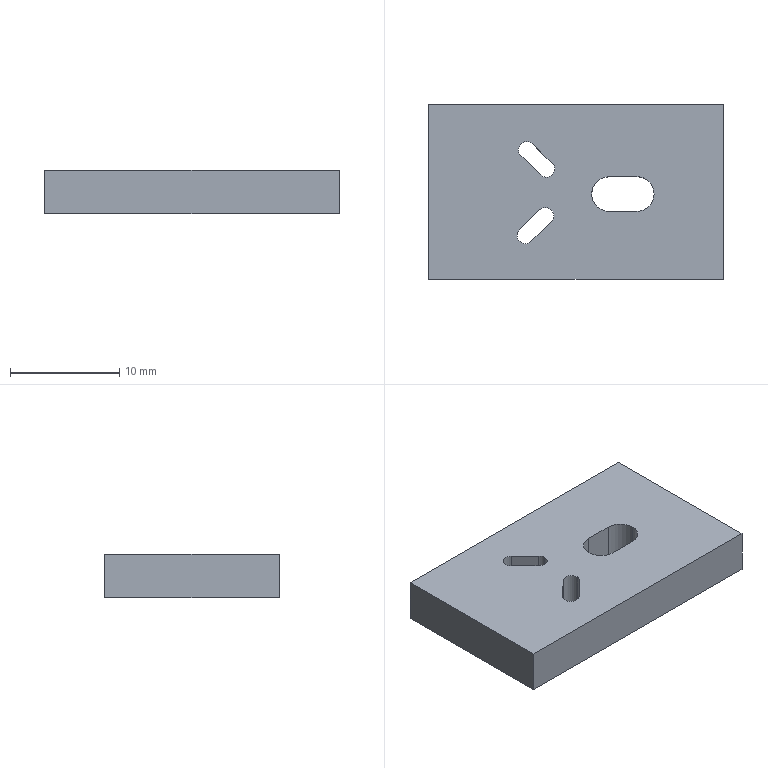Part | SolidWorks | features Cut 2, Extrusion 1 | 1 solid | 21 faces | box 27 x 16 x 4 mm | volume 1619 mm3 | plane 12 | cylinder 9 | commonest cylinder face diameters 1.5 x6 3.18 x3
STEP:
#1=CARTESIAN_POINT('',(9.464,-2.48,0.));
#2=VERTEX_POINT('',#1);
#3=CARTESIAN_POINT('',(11.055,-4.07,0.));
#4=VERTEX_POINT('',#3);
#5=CARTESIAN_POINT('',(9.465,-4.07,0.));
#6=DIRECTION('',(0.,0.,-1.));
#7=DIRECTION('',(1.,0.,0.));
#8=AXIS2_PLACEMENT_3D('',#5,#6,#7);
#9=CIRCLE('',#8,1.59);
#10=EDGE_CURVE('',#2,#4,#9,.T.);
#11=ORIENTED_EDGE('',*,*,#10,.T.);
#12=CARTESIAN_POINT('',(11.055,-4.07,4.));
#13=VERTEX_POINT('',#12);
#14=CARTESIAN_POINT('',(11.055,-4.07,-4.497));
#15=DIRECTION('',(0.,0.,1.));
#16=VECTOR('',#15,1000.);
#17=LINE('',#14,#16);
#18=EDGE_CURVE('',#4,#13,#17,.T.);
#19=ORIENTED_EDGE('',*,*,#18,.T.);
#20=CARTESIAN_POINT('',(9.464,-2.48,4.));
#21=VERTEX_POINT('',#20);
#22=CARTESIAN_POINT('',(9.465,-4.07,4.));
#23=DIRECTION('',(0.,0.,1.));
#24=DIRECTION('',(1.,0.,0.));
#25=AXIS2_PLACEMENT_3D('',#22,#23,#24);
#26=CIRCLE('',#25,1.59);
#27=EDGE_CURVE('',#13,#21,#26,.T.);
#28=ORIENTED_EDGE('',*,*,#27,.T.);
#29=CARTESIAN_POINT('',(9.464,-2.48,-5.208));
#30=DIRECTION('',(0.,0.,1.));
#31=VECTOR('',#30,1000.);
#32=LINE('',#29,#31);
#33=EDGE_CURVE('',#2,#21,#32,.T.);
#34=ORIENTED_EDGE('',*,*,#33,.F.);
#35=EDGE_LOOP('',(#11,#19,#28,#34));
#36=FACE_OUTER_BOUND('',#35,.T.);
#37=CARTESIAN_POINT('',(9.465,-4.07,-4.497));
#38=DIRECTION('',(0.,0.,1.));
#39=DIRECTION('',(1.,0.,0.));
#40=AXIS2_PLACEMENT_3D('',#37,#38,#39);
#41=CYLINDRICAL_SURFACE('',#40,1.59);
#42=ADVANCED_FACE('',(#36),#41,.F.);
#43=CARTESIAN_POINT('',(1.721,-1.242,0.));
#44=VERTEX_POINT('',#43);
#45=CARTESIAN_POINT('',(1.95,-1.782,0.));
#46=VERTEX_POINT('',#45);
#47=CARTESIAN_POINT('',(1.2,-1.782,0.));
#48=DIRECTION('',(0.,0.,-1.));
#49=DIRECTION('',(1.,0.,0.));
#50=AXIS2_PLACEMENT_3D('',#47,#48,#49);
#51=CIRCLE('',#50,0.75);
#52=EDGE_CURVE('',#44,#46,#51,.T.);
#53=ORIENTED_EDGE('',*,*,#52,.T.);
#54=CARTESIAN_POINT('',(1.95,-1.782,4.));
#55=VERTEX_POINT('',#54);
#56=CARTESIAN_POINT('',(1.95,-1.782,-4.497));
#57=DIRECTION('',(0.,0.,1.));
#58=VECTOR('',#57,1000.);
#59=LINE('',#56,#58);
#60=EDGE_CURVE('',#46,#55,#59,.T.);
#61=ORIENTED_EDGE('',*,*,#60,.T.);
#62=CARTESIAN_POINT('',(1.721,-1.242,4.));
#63=VERTEX_POINT('',#62);
#64=CARTESIAN_POINT('',(1.2,-1.782,4.));
#65=DIRECTION('',(0.,0.,1.));
#66=DIRECTION('',(1.,0.,0.));
#67=AXIS2_PLACEMENT_3D('',#64,#65,#66);
#68=CIRCLE('',#67,0.75);
#69=EDGE_CURVE('',#55,#63,#68,.T.);
#70=ORIENTED_EDGE('',*,*,#69,.T.);
#71=CARTESIAN_POINT('',(1.721,-1.242,-5.208));
#72=DIRECTION('',(0.,0.,1.));
#73=VECTOR('',#72,1000.);
#74=LINE('',#71,#73);
#75=EDGE_CURVE('',#44,#63,#74,.T.);
#76=ORIENTED_EDGE('',*,*,#75,.F.);
#77=EDGE_LOOP('',(#53,#61,#70,#76));
#78=FACE_OUTER_BOUND('',#77,.T.);
#79=CARTESIAN_POINT('',(1.2,-1.782,-4.497));
#80=DIRECTION('',(0.,0.,1.));
#81=DIRECTION('',(1.,0.,0.));
#82=AXIS2_PLACEMENT_3D('',#79,#80,#81);
#83=CYLINDRICAL_SURFACE('',#82,0.75);
#84=ADVANCED_FACE('',(#78),#83,.F.);
#85=CARTESIAN_POINT('',(0.6012,-5.518,0.));
#86=VERTEX_POINT('',#85);
#87=CARTESIAN_POINT('',(1.873,-6.057,0.));
#88=VERTEX_POINT('',#87);
#89=CARTESIAN_POINT('',(1.123,-6.057,0.));
#90=DIRECTION('',(0.,0.,-1.));
#91=DIRECTION('',(1.,0.,0.));
#92=AXIS2_PLACEMENT_3D('',#89,#90,#91);
#93=CIRCLE('',#92,0.75);
#94=EDGE_CURVE('',#86,#88,#93,.T.);
#95=ORIENTED_EDGE('',*,*,#94,.T.);
#96=CARTESIAN_POINT('',(1.873,-6.057,4.));
#97=VERTEX_POINT('',#96);
#98=CARTESIAN_POINT('',(1.873,-6.057,-4.497));
#99=DIRECTION('',(0.,0.,1.));
#100=VECTOR('',#99,1000.);
#101=LINE('',#98,#100);
#102=EDGE_CURVE('',#88,#97,#101,.T.);
#103=ORIENTED_EDGE('',*,*,#102,.T.);
#104=CARTESIAN_POINT('',(0.6012,-5.518,4.));
#105=VERTEX_POINT('',#104);
#106=CARTESIAN_POINT('',(1.123,-6.057,4.));
#107=DIRECTION('',(0.,0.,1.));
#108=DIRECTION('',(1.,0.,0.));
#109=AXIS2_PLACEMENT_3D('',#106,#107,#108);
#110=CIRCLE('',#109,0.75);
#111=EDGE_CURVE('',#97,#105,#110,.T.);
#112=ORIENTED_EDGE('',*,*,#111,.T.);
#113=CARTESIAN_POINT('',(0.6012,-5.518,-5.208));
#114=DIRECTION('',(0.,0.,1.));
#115=VECTOR('',#114,1000.);
#116=LINE('',#113,#115);
#117=EDGE_CURVE('',#86,#105,#116,.T.);
#118=ORIENTED_EDGE('',*,*,#117,.F.);
#119=EDGE_LOOP('',(#95,#103,#112,#118));
#120=FACE_OUTER_BOUND('',#119,.T.);
#121=CARTESIAN_POINT('',(1.123,-6.057,-4.497));
#122=DIRECTION('',(0.,0.,1.));
#123=DIRECTION('',(1.,0.,0.));
#124=AXIS2_PLACEMENT_3D('',#121,#122,#123);
#125=CYLINDRICAL_SURFACE('',#124,0.75);
#126=ADVANCED_FACE('',(#120),#125,.F.);
#127=ORIENTED_EDGE('',*,*,#102,.F.);
#128=CARTESIAN_POINT('',(1.644,-6.596,0.));
#129=VERTEX_POINT('',#128);
#130=CARTESIAN_POINT('',(1.123,-6.057,0.));
#131=DIRECTION('',(0.,0.,-1.));
#132=DIRECTION('',(1.,0.,0.));
#133=AXIS2_PLACEMENT_3D('',#130,#131,#132);
#134=CIRCLE('',#133,0.75);
#135=EDGE_CURVE('',#88,#129,#134,.T.);
#136=ORIENTED_EDGE('',*,*,#135,.T.);
#137=CARTESIAN_POINT('',(1.644,-6.596,4.));
#138=VERTEX_POINT('',#137);
#139=CARTESIAN_POINT('',(1.644,-6.596,-5.208));
#140=DIRECTION('',(0.,0.,1.));
#141=VECTOR('',#140,1000.);
#142=LINE('',#139,#141);
#143=EDGE_CURVE('',#129,#138,#142,.T.);
#144=ORIENTED_EDGE('',*,*,#143,.T.);
#145=CARTESIAN_POINT('',(1.123,-6.057,4.));
#146=DIRECTION('',(0.,0.,1.));
#147=DIRECTION('',(1.,0.,0.));
#148=AXIS2_PLACEMENT_3D('',#145,#146,#147);
#149=CIRCLE('',#148,0.75);
#150=EDGE_CURVE('',#138,#97,#149,.T.);
#151=ORIENTED_EDGE('',*,*,#150,.T.);
#152=EDGE_LOOP('',(#127,#136,#144,#151));
#153=FACE_OUTER_BOUND('',#152,.T.);
#154=CARTESIAN_POINT('',(1.123,-6.057,-4.497));
#155=DIRECTION('',(0.,0.,1.));
#156=DIRECTION('',(1.,0.,0.));
#157=AXIS2_PLACEMENT_3D('',#154,#155,#156);
#158=CYLINDRICAL_SURFACE('',#157,0.75);
#159=ADVANCED_FACE('',(#153),#158,.F.);
#160=CARTESIAN_POINT('',(-9.601,4.118,0.));
#161=VERTEX_POINT('',#160);
#162=CARTESIAN_POINT('',(-9.601,-11.882,0.));
#163=VERTEX_POINT('',#162);
#164=CARTESIAN_POINT('',(-9.601,4.118,0.));
#165=DIRECTION('',(0.,-1.,0.));
#166=VECTOR('',#165,1000.);
#167=LINE('',#164,#166);
#168=EDGE_CURVE('',#161,#163,#167,.T.);
#169=ORIENTED_EDGE('',*,*,#168,.T.);
#170=CARTESIAN_POINT('',(-9.601,-11.882,4.));
#171=VERTEX_POINT('',#170);
#172=CARTESIAN_POINT('',(-9.601,-11.882,4.));
#173=DIRECTION('',(0.,0.,-1.));
#174=VECTOR('',#173,1000.);
#175=LINE('',#172,#174);
#176=EDGE_CURVE('',#171,#163,#175,.T.);
#177=ORIENTED_EDGE('',*,*,#176,.F.);
#178=CARTESIAN_POINT('',(-9.601,4.118,4.));
#179=VERTEX_POINT('',#178);
#180=CARTESIAN_POINT('',(-9.601,4.118,4.));
#181=DIRECTION('',(0.,-1.,0.));
#182=VECTOR('',#181,1000.);
#183=LINE('',#180,#182);
#184=EDGE_CURVE('',#179,#171,#183,.T.);
#185=ORIENTED_EDGE('',*,*,#184,.F.);
#186=CARTESIAN_POINT('',(-9.601,4.118,4.));
#187=DIRECTION('',(0.,0.,-1.));
#188=VECTOR('',#187,1000.);
#189=LINE('',#186,#188);
#190=EDGE_CURVE('',#179,#161,#189,.T.);
#191=ORIENTED_EDGE('',*,*,#190,.T.);
#192=EDGE_LOOP('',(#169,#177,#185,#191));
#193=FACE_OUTER_BOUND('',#192,.T.);
#194=CARTESIAN_POINT('',(-9.601,4.118,4.));
#195=DIRECTION('',(1.,0.,0.));
#196=DIRECTION('',(0.,1.,0.));
#197=AXIS2_PLACEMENT_3D('',#194,#195,#196);
#198=PLANE('',#197);
#199=ADVANCED_FACE('',(#193),#198,.F.);
#200=CARTESIAN_POINT('',(17.399,-11.882,0.));
#201=VERTEX_POINT('',#200);
#202=CARTESIAN_POINT('',(-9.601,-11.882,0.));
#203=DIRECTION('',(1.,0.,0.));
#204=VECTOR('',#203,1000.);
#205=LINE('',#202,#204);
#206=EDGE_CURVE('',#163,#201,#205,.T.);
#207=ORIENTED_EDGE('',*,*,#206,.T.);
#208=CARTESIAN_POINT('',(17.399,-11.882,4.));
#209=VERTEX_POINT('',#208);
#210=CARTESIAN_POINT('',(17.399,-11.882,4.));
#211=DIRECTION('',(0.,0.,-1.));
#212=VECTOR('',#211,1000.);
#213=LINE('',#210,#212);
#214=EDGE_CURVE('',#209,#201,#213,.T.);
#215=ORIENTED_EDGE('',*,*,#214,.F.);
#216=CARTESIAN_POINT('',(-9.601,-11.882,4.));
#217=DIRECTION('',(1.,0.,0.));
#218=VECTOR('',#217,1000.);
#219=LINE('',#216,#218);
#220=EDGE_CURVE('',#171,#209,#219,.T.);
#221=ORIENTED_EDGE('',*,*,#220,.F.);
#222=ORIENTED_EDGE('',*,*,#176,.T.);
#223=EDGE_LOOP('',(#207,#215,#221,#222));
#224=FACE_OUTER_BOUND('',#223,.T.);
#225=CARTESIAN_POINT('',(-9.601,-11.882,4.));
#226=DIRECTION('',(0.,1.,0.));
#227=DIRECTION('',(0.,0.,1.));
#228=AXIS2_PLACEMENT_3D('',#225,#226,#227);
#229=PLANE('',#228);
#230=ADVANCED_FACE('',(#224),#229,.F.);
#231=CARTESIAN_POINT('',(17.399,4.118,0.));
#232=VERTEX_POINT('',#231);
#233=CARTESIAN_POINT('',(17.399,4.118,0.));
#234=DIRECTION('',(0.,1.,0.));
#235=VECTOR('',#234,1000.);
#236=LINE('',#233,#235);
#237=EDGE_CURVE('',#201,#232,#236,.T.);
#238=ORIENTED_EDGE('',*,*,#237,.T.);
#239=CARTESIAN_POINT('',(17.399,4.118,4.));
#240=VERTEX_POINT('',#239);
#241=CARTESIAN_POINT('',(17.399,4.118,4.));
#242=DIRECTION('',(0.,0.,-1.));
#243=VECTOR('',#242,1000.);
#244=LINE('',#241,#243);
#245=EDGE_CURVE('',#240,#232,#244,.T.);
#246=ORIENTED_EDGE('',*,*,#245,.F.);
#247=CARTESIAN_POINT('',(17.399,4.118,4.));
#248=DIRECTION('',(0.,1.,0.));
#249=VECTOR('',#248,1000.);
#250=LINE('',#247,#249);
#251=EDGE_CURVE('',#209,#240,#250,.T.);
#252=ORIENTED_EDGE('',*,*,#251,.F.);
#253=ORIENTED_EDGE('',*,*,#214,.T.);
#254=EDGE_LOOP('',(#238,#246,#252,#253));
#255=FACE_OUTER_BOUND('',#254,.T.);
#256=CARTESIAN_POINT('',(17.399,4.118,4.));
#257=DIRECTION('',(-1.,0.,0.));
#258=DIRECTION('',(0.,-1.,0.));
#259=AXIS2_PLACEMENT_3D('',#256,#257,#258);
#260=PLANE('',#259);
#261=ADVANCED_FACE('',(#255),#260,.F.);
#262=CARTESIAN_POINT('',(-9.601,4.118,0.));
#263=DIRECTION('',(-1.,0.,0.));
#264=VECTOR('',#263,1000.);
#265=LINE('',#262,#264);
#266=EDGE_CURVE('',#232,#161,#265,.T.);
#267=ORIENTED_EDGE('',*,*,#266,.T.);
#268=ORIENTED_EDGE('',*,*,#190,.F.);
#269=CARTESIAN_POINT('',(-9.601,4.118,4.));
#270=DIRECTION('',(-1.,0.,0.));
#271=VECTOR('',#270,1000.);
#272=LINE('',#269,#271);
#273=EDGE_CURVE('',#240,#179,#272,.T.);
#274=ORIENTED_EDGE('',*,*,#273,.F.);
#275=ORIENTED_EDGE('',*,*,#245,.T.);
#276=EDGE_LOOP('',(#267,#268,#274,#275));
#277=FACE_OUTER_BOUND('',#276,.T.);
#278=CARTESIAN_POINT('',(-9.601,4.118,4.));
#279=DIRECTION('',(0.,-1.,0.));
#280=DIRECTION('',(0.,0.,-1.));
#281=AXIS2_PLACEMENT_3D('',#278,#279,#280);
#282=PLANE('',#281);
#283=ADVANCED_FACE('',(#277),#282,.F.);
#284=CARTESIAN_POINT('',(-0.1034,0.5215,4.));
#285=VERTEX_POINT('',#284);
#286=CARTESIAN_POINT('',(1.721,-1.242,4.));
#287=DIRECTION('',(-0.719,0.695,0.));
#288=VECTOR('',#287,1000.);
#289=LINE('',#286,#288);
#290=EDGE_CURVE('',#63,#285,#289,.T.);
#291=ORIENTED_EDGE('',*,*,#290,.F.);
#292=ORIENTED_EDGE('',*,*,#69,.F.);
#293=CARTESIAN_POINT('',(0.6786,-2.321,4.));
#294=VERTEX_POINT('',#293);
#295=CARTESIAN_POINT('',(1.2,-1.782,4.));
#296=DIRECTION('',(0.,0.,1.));
#297=DIRECTION('',(1.,0.,0.));
#298=AXIS2_PLACEMENT_3D('',#295,#296,#297);
#299=CIRCLE('',#298,0.75);
#300=EDGE_CURVE('',#294,#55,#299,.T.);
#301=ORIENTED_EDGE('',*,*,#300,.F.);
#302=CARTESIAN_POINT('',(-1.146,-0.5569,4.));
#303=VERTEX_POINT('',#302);
#304=CARTESIAN_POINT('',(-1.146,-0.5569,4.));
#305=DIRECTION('',(0.719,-0.695,0.));
#306=VECTOR('',#305,1000.);
#307=LINE('',#304,#306);
#308=EDGE_CURVE('',#303,#294,#307,.T.);
#309=ORIENTED_EDGE('',*,*,#308,.F.);
#310=CARTESIAN_POINT('',(-0.6247,-0.01768,4.));
#311=DIRECTION('',(0.,0.,1.));
#312=DIRECTION('',(1.,0.,0.));
#313=AXIS2_PLACEMENT_3D('',#310,#311,#312);
#314=CIRCLE('',#313,0.75);
#315=EDGE_CURVE('',#285,#303,#314,.T.);
#316=ORIENTED_EDGE('',*,*,#315,.F.);
#317=EDGE_LOOP('',(#291,#292,#301,#309,#316));
#318=FACE_BOUND('',#317,.T.);
#319=CARTESIAN_POINT('',(6.932,-2.481,4.));
#320=VERTEX_POINT('',#319);
#321=CARTESIAN_POINT('',(6.932,-2.481,4.));
#322=DIRECTION('',(-1.,-0.0007677,0.));
#323=VECTOR('',#322,1000.);
#324=LINE('',#321,#323);
#325=EDGE_CURVE('',#21,#320,#324,.T.);
#326=ORIENTED_EDGE('',*,*,#325,.F.);
#327=ORIENTED_EDGE('',*,*,#27,.F.);
#328=CARTESIAN_POINT('',(9.467,-5.66,4.));
#329=VERTEX_POINT('',#328);
#330=CARTESIAN_POINT('',(9.465,-4.07,4.));
#331=DIRECTION('',(0.,0.,1.));
#332=DIRECTION('',(1.,0.,0.));
#333=AXIS2_PLACEMENT_3D('',#330,#331,#332);
#334=CIRCLE('',#333,1.59);
#335=EDGE_CURVE('',#329,#13,#334,.T.);
#336=ORIENTED_EDGE('',*,*,#335,.F.);
#337=CARTESIAN_POINT('',(6.934,-5.661,4.));
#338=VERTEX_POINT('',#337);
#339=CARTESIAN_POINT('',(6.934,-5.661,4.));
#340=DIRECTION('',(1.,0.0007677,0.));
#341=VECTOR('',#340,1000.);
#342=LINE('',#339,#341);
#343=EDGE_CURVE('',#338,#329,#342,.T.);
#344=ORIENTED_EDGE('',*,*,#343,.F.);
#345=CARTESIAN_POINT('',(6.933,-4.071,4.));
#346=DIRECTION('',(0.,0.,1.));
#347=DIRECTION('',(1.,0.,0.));
#348=AXIS2_PLACEMENT_3D('',#345,#346,#347);
#349=CIRCLE('',#348,1.59);
#350=EDGE_CURVE('',#320,#338,#349,.T.);
#351=ORIENTED_EDGE('',*,*,#350,.F.);
#352=EDGE_LOOP('',(#326,#327,#336,#344,#351));
#353=FACE_BOUND('',#352,.T.);
#354=CARTESIAN_POINT('',(-0.2339,-8.411,4.));
#355=VERTEX_POINT('',#354);
#356=CARTESIAN_POINT('',(1.644,-6.596,4.));
#357=DIRECTION('',(0.719,0.695,0.));
#358=VECTOR('',#357,1000.);
#359=LINE('',#356,#358);
#360=EDGE_CURVE('',#355,#138,#359,.T.);
#361=ORIENTED_EDGE('',*,*,#360,.F.);
#362=CARTESIAN_POINT('',(-1.276,-7.333,4.));
#363=VERTEX_POINT('',#362);
#364=CARTESIAN_POINT('',(-0.7552,-7.872,4.));
#365=DIRECTION('',(0.,0.,1.));
#366=DIRECTION('',(1.,0.,0.));
#367=AXIS2_PLACEMENT_3D('',#364,#365,#366);
#368=CIRCLE('',#367,0.75);
#369=EDGE_CURVE('',#363,#355,#368,.T.);
#370=ORIENTED_EDGE('',*,*,#369,.F.);
#371=CARTESIAN_POINT('',(-1.276,-7.333,4.));
#372=DIRECTION('',(-0.719,-0.695,0.));
#373=VECTOR('',#372,1000.);
#374=LINE('',#371,#373);
#375=EDGE_CURVE('',#105,#363,#374,.T.);
#376=ORIENTED_EDGE('',*,*,#375,.F.);
#377=ORIENTED_EDGE('',*,*,#111,.F.);
#378=ORIENTED_EDGE('',*,*,#150,.F.);
#379=EDGE_LOOP('',(#361,#370,#376,#377,#378));
#380=FACE_BOUND('',#379,.T.);
#381=ORIENTED_EDGE('',*,*,#184,.T.);
#382=ORIENTED_EDGE('',*,*,#220,.T.);
#383=ORIENTED_EDGE('',*,*,#251,.T.);
#384=ORIENTED_EDGE('',*,*,#273,.T.);
#385=EDGE_LOOP('',(#381,#382,#383,#384));
#386=FACE_OUTER_BOUND('',#385,.T.);
#387=CARTESIAN_POINT('',(0.,0.,4.));
#388=DIRECTION('',(0.,0.,1.));
#389=DIRECTION('',(1.,0.,0.));
#390=AXIS2_PLACEMENT_3D('',#387,#388,#389);
#391=PLANE('',#390);
#392=ADVANCED_FACE('',(#318,#353,#380,#386),#391,.T.);
#393=ORIENTED_EDGE('',*,*,#10,.F.);
#394=CARTESIAN_POINT('',(6.932,-2.481,0.));
#395=VERTEX_POINT('',#394);
#396=CARTESIAN_POINT('',(6.932,-2.481,0.));
#397=DIRECTION('',(1.,0.0007677,0.));
#398=VECTOR('',#397,1000.);
#399=LINE('',#396,#398);
#400=EDGE_CURVE('',#395,#2,#399,.T.);
#401=ORIENTED_EDGE('',*,*,#400,.F.);
#402=CARTESIAN_POINT('',(6.934,-5.661,0.));
#403=VERTEX_POINT('',#402);
#404=CARTESIAN_POINT('',(6.933,-4.071,0.));
#405=DIRECTION('',(0.,0.,-1.));
#406=DIRECTION('',(1.,0.,0.));
#407=AXIS2_PLACEMENT_3D('',#404,#405,#406);
#408=CIRCLE('',#407,1.59);
#409=EDGE_CURVE('',#403,#395,#408,.T.);
#410=ORIENTED_EDGE('',*,*,#409,.F.);
#411=CARTESIAN_POINT('',(9.467,-5.66,0.));
#412=VERTEX_POINT('',#411);
#413=CARTESIAN_POINT('',(6.934,-5.661,0.));
#414=DIRECTION('',(-1.,-0.0007677,0.));
#415=VECTOR('',#414,1000.);
#416=LINE('',#413,#415);
#417=EDGE_CURVE('',#412,#403,#416,.T.);
#418=ORIENTED_EDGE('',*,*,#417,.F.);
#419=CARTESIAN_POINT('',(9.465,-4.07,0.));
#420=DIRECTION('',(0.,0.,-1.));
#421=DIRECTION('',(1.,0.,0.));
#422=AXIS2_PLACEMENT_3D('',#419,#420,#421);
#423=CIRCLE('',#422,1.59);
#424=EDGE_CURVE('',#4,#412,#423,.T.);
#425=ORIENTED_EDGE('',*,*,#424,.F.);
#426=EDGE_LOOP('',(#393,#401,#410,#418,#425));
#427=FACE_BOUND('',#426,.T.);
#428=CARTESIAN_POINT('',(-0.2339,-8.411,0.));
#429=VERTEX_POINT('',#428);
#430=CARTESIAN_POINT('',(-1.276,-7.333,0.));
#431=VERTEX_POINT('',#430);
#432=CARTESIAN_POINT('',(-0.7552,-7.872,0.));
#433=DIRECTION('',(0.,0.,-1.));
#434=DIRECTION('',(1.,0.,0.));
#435=AXIS2_PLACEMENT_3D('',#432,#433,#434);
#436=CIRCLE('',#435,0.75);
#437=EDGE_CURVE('',#429,#431,#436,.T.);
#438=ORIENTED_EDGE('',*,*,#437,.F.);
#439=CARTESIAN_POINT('',(1.644,-6.596,0.));
#440=DIRECTION('',(-0.719,-0.695,0.));
#441=VECTOR('',#440,1000.);
#442=LINE('',#439,#441);
#443=EDGE_CURVE('',#129,#429,#442,.T.);
#444=ORIENTED_EDGE('',*,*,#443,.F.);
#445=ORIENTED_EDGE('',*,*,#135,.F.);
#446=ORIENTED_EDGE('',*,*,#94,.F.);
#447=CARTESIAN_POINT('',(-1.276,-7.333,0.));
#448=DIRECTION('',(0.719,0.695,0.));
#449=VECTOR('',#448,1000.);
#450=LINE('',#447,#449);
#451=EDGE_CURVE('',#431,#86,#450,.T.);
#452=ORIENTED_EDGE('',*,*,#451,.F.);
#453=EDGE_LOOP('',(#438,#444,#445,#446,#452));
#454=FACE_BOUND('',#453,.T.);
#455=ORIENTED_EDGE('',*,*,#52,.F.);
#456=CARTESIAN_POINT('',(-0.1034,0.5215,0.));
#457=VERTEX_POINT('',#456);
#458=CARTESIAN_POINT('',(1.721,-1.242,0.));
#459=DIRECTION('',(0.719,-0.695,0.));
#460=VECTOR('',#459,1000.);
#461=LINE('',#458,#460);
#462=EDGE_CURVE('',#457,#44,#461,.T.);
#463=ORIENTED_EDGE('',*,*,#462,.F.);
#464=CARTESIAN_POINT('',(-1.146,-0.5569,0.));
#465=VERTEX_POINT('',#464);
#466=CARTESIAN_POINT('',(-0.6247,-0.01768,0.));
#467=DIRECTION('',(0.,0.,-1.));
#468=DIRECTION('',(1.,0.,0.));
#469=AXIS2_PLACEMENT_3D('',#466,#467,#468);
#470=CIRCLE('',#469,0.75);
#471=EDGE_CURVE('',#465,#457,#470,.T.);
#472=ORIENTED_EDGE('',*,*,#471,.F.);
#473=CARTESIAN_POINT('',(0.6786,-2.321,0.));
#474=VERTEX_POINT('',#473);
#475=CARTESIAN_POINT('',(-1.146,-0.5569,0.));
#476=DIRECTION('',(-0.719,0.695,0.));
#477=VECTOR('',#476,1000.);
#478=LINE('',#475,#477);
#479=EDGE_CURVE('',#474,#465,#478,.T.);
#480=ORIENTED_EDGE('',*,*,#479,.F.);
#481=CARTESIAN_POINT('',(1.2,-1.782,0.));
#482=DIRECTION('',(0.,0.,-1.));
#483=DIRECTION('',(1.,0.,0.));
#484=AXIS2_PLACEMENT_3D('',#481,#482,#483);
#485=CIRCLE('',#484,0.75);
#486=EDGE_CURVE('',#46,#474,#485,.T.);
#487=ORIENTED_EDGE('',*,*,#486,.F.);
#488=EDGE_LOOP('',(#455,#463,#472,#480,#487));
#489=FACE_BOUND('',#488,.T.);
#490=ORIENTED_EDGE('',*,*,#168,.F.);
#491=ORIENTED_EDGE('',*,*,#266,.F.);
#492=ORIENTED_EDGE('',*,*,#237,.F.);
#493=ORIENTED_EDGE('',*,*,#206,.F.);
#494=EDGE_LOOP('',(#490,#491,#492,#493));
#495=FACE_OUTER_BOUND('',#494,.T.);
#496=CARTESIAN_POINT('',(0.,0.,0.));
#497=DIRECTION('',(0.,0.,1.));
#498=DIRECTION('',(1.,0.,0.));
#499=AXIS2_PLACEMENT_3D('',#496,#497,#498);
#500=PLANE('',#499);
#501=ADVANCED_FACE('',(#427,#454,#489,#495),#500,.F.);
#502=ORIENTED_EDGE('',*,*,#60,.F.);
#503=ORIENTED_EDGE('',*,*,#486,.T.);
#504=CARTESIAN_POINT('',(0.6786,-2.321,-5.208));
#505=DIRECTION('',(0.,0.,1.));
#506=VECTOR('',#505,1000.);
#507=LINE('',#504,#506);
#508=EDGE_CURVE('',#474,#294,#507,.T.);
#509=ORIENTED_EDGE('',*,*,#508,.T.);
#510=ORIENTED_EDGE('',*,*,#300,.T.);
#511=EDGE_LOOP('',(#502,#503,#509,#510));
#512=FACE_OUTER_BOUND('',#511,.T.);
#513=CARTESIAN_POINT('',(1.2,-1.782,-4.497));
#514=DIRECTION('',(0.,0.,1.));
#515=DIRECTION('',(1.,0.,0.));
#516=AXIS2_PLACEMENT_3D('',#513,#514,#515);
#517=CYLINDRICAL_SURFACE('',#516,0.75);
#518=ADVANCED_FACE('',(#512),#517,.F.);
#519=ORIENTED_EDGE('',*,*,#18,.F.);
#520=ORIENTED_EDGE('',*,*,#424,.T.);
#521=CARTESIAN_POINT('',(9.467,-5.66,-5.208));
#522=DIRECTION('',(0.,0.,1.));
#523=VECTOR('',#522,1000.);
#524=LINE('',#521,#523);
#525=EDGE_CURVE('',#412,#329,#524,.T.);
#526=ORIENTED_EDGE('',*,*,#525,.T.);
#527=ORIENTED_EDGE('',*,*,#335,.T.);
#528=EDGE_LOOP('',(#519,#520,#526,#527));
#529=FACE_OUTER_BOUND('',#528,.T.);
#530=CARTESIAN_POINT('',(9.465,-4.07,-4.497));
#531=DIRECTION('',(0.,0.,1.));
#532=DIRECTION('',(1.,0.,0.));
#533=AXIS2_PLACEMENT_3D('',#530,#531,#532);
#534=CYLINDRICAL_SURFACE('',#533,1.59);
#535=ADVANCED_FACE('',(#529),#534,.F.);
#536=ORIENTED_EDGE('',*,*,#409,.T.);
#537=CARTESIAN_POINT('',(6.932,-2.481,-5.208));
#538=DIRECTION('',(0.,0.,1.));
#539=VECTOR('',#538,1000.);
#540=LINE('',#537,#539);
#541=EDGE_CURVE('',#395,#320,#540,.T.);
#542=ORIENTED_EDGE('',*,*,#541,.T.);
#543=ORIENTED_EDGE('',*,*,#350,.T.);
#544=CARTESIAN_POINT('',(6.934,-5.661,-5.208));
#545=DIRECTION('',(0.,0.,1.));
#546=VECTOR('',#545,1000.);
#547=LINE('',#544,#546);
#548=EDGE_CURVE('',#403,#338,#547,.T.);
#549=ORIENTED_EDGE('',*,*,#548,.F.);
#550=EDGE_LOOP('',(#536,#542,#543,#549));
#551=FACE_OUTER_BOUND('',#550,.T.);
#552=CARTESIAN_POINT('',(6.933,-4.071,-5.208));
#553=DIRECTION('',(0.,0.,1.));
#554=DIRECTION('',(1.,0.,0.));
#555=AXIS2_PLACEMENT_3D('',#552,#553,#554);
#556=CYLINDRICAL_SURFACE('',#555,1.59);
#557=ADVANCED_FACE('',(#551),#556,.F.);
#558=ORIENTED_EDGE('',*,*,#400,.T.);
#559=ORIENTED_EDGE('',*,*,#33,.T.);
#560=ORIENTED_EDGE('',*,*,#325,.T.);
#561=ORIENTED_EDGE('',*,*,#541,.F.);
#562=EDGE_LOOP('',(#558,#559,#560,#561));
#563=FACE_OUTER_BOUND('',#562,.T.);
#564=CARTESIAN_POINT('',(6.932,-2.481,-5.208));
#565=DIRECTION('',(-0.0007677,1.,0.));
#566=DIRECTION('',(-1.,-0.0007677,0.));
#567=AXIS2_PLACEMENT_3D('',#564,#565,#566);
#568=PLANE('',#567);
#569=ADVANCED_FACE('',(#563),#568,.F.);
#570=ORIENTED_EDGE('',*,*,#417,.T.);
#571=ORIENTED_EDGE('',*,*,#548,.T.);
#572=ORIENTED_EDGE('',*,*,#343,.T.);
#573=ORIENTED_EDGE('',*,*,#525,.F.);
#574=EDGE_LOOP('',(#570,#571,#572,#573));
#575=FACE_OUTER_BOUND('',#574,.T.);
#576=CARTESIAN_POINT('',(6.934,-5.661,-5.208));
#577=DIRECTION('',(0.0007677,-1.,0.));
#578=DIRECTION('',(1.,0.0007677,0.));
#579=AXIS2_PLACEMENT_3D('',#576,#577,#578);
#580=PLANE('',#579);
#581=ADVANCED_FACE('',(#575),#580,.F.);
#582=ORIENTED_EDGE('',*,*,#443,.T.);
#583=CARTESIAN_POINT('',(-0.2339,-8.411,-5.208));
#584=DIRECTION('',(0.,0.,1.));
#585=VECTOR('',#584,1000.);
#586=LINE('',#583,#585);
#587=EDGE_CURVE('',#429,#355,#586,.T.);
#588=ORIENTED_EDGE('',*,*,#587,.T.);
#589=ORIENTED_EDGE('',*,*,#360,.T.);
#590=ORIENTED_EDGE('',*,*,#143,.F.);
#591=EDGE_LOOP('',(#582,#588,#589,#590));
#592=FACE_OUTER_BOUND('',#591,.T.);
#593=CARTESIAN_POINT('',(1.644,-6.596,-5.208));
#594=DIRECTION('',(0.695,-0.719,0.));
#595=DIRECTION('',(0.719,0.695,0.));
#596=AXIS2_PLACEMENT_3D('',#593,#594,#595);
#597=PLANE('',#596);
#598=ADVANCED_FACE('',(#592),#597,.F.);
#599=ORIENTED_EDGE('',*,*,#437,.T.);
#600=CARTESIAN_POINT('',(-1.276,-7.333,-5.208));
#601=DIRECTION('',(0.,0.,1.));
#602=VECTOR('',#601,1000.);
#603=LINE('',#600,#602);
#604=EDGE_CURVE('',#431,#363,#603,.T.);
#605=ORIENTED_EDGE('',*,*,#604,.T.);
#606=ORIENTED_EDGE('',*,*,#369,.T.);
#607=ORIENTED_EDGE('',*,*,#587,.F.);
#608=EDGE_LOOP('',(#599,#605,#606,#607));
#609=FACE_OUTER_BOUND('',#608,.T.);
#610=CARTESIAN_POINT('',(-0.7552,-7.872,-5.208));
#611=DIRECTION('',(0.,0.,1.));
#612=DIRECTION('',(1.,0.,0.));
#613=AXIS2_PLACEMENT_3D('',#610,#611,#612);
#614=CYLINDRICAL_SURFACE('',#613,0.75);
#615=ADVANCED_FACE('',(#609),#614,.F.);
#616=ORIENTED_EDGE('',*,*,#451,.T.);
#617=ORIENTED_EDGE('',*,*,#117,.T.);
#618=ORIENTED_EDGE('',*,*,#375,.T.);
#619=ORIENTED_EDGE('',*,*,#604,.F.);
#620=EDGE_LOOP('',(#616,#617,#618,#619));
#621=FACE_OUTER_BOUND('',#620,.T.);
#622=CARTESIAN_POINT('',(-1.276,-7.333,-5.208));
#623=DIRECTION('',(-0.695,0.719,0.));
#624=DIRECTION('',(-0.719,-0.695,0.));
#625=AXIS2_PLACEMENT_3D('',#622,#623,#624);
#626=PLANE('',#625);
#627=ADVANCED_FACE('',(#621),#626,.F.);
#628=ORIENTED_EDGE('',*,*,#471,.T.);
#629=CARTESIAN_POINT('',(-0.1034,0.5215,-5.208));
#630=DIRECTION('',(0.,0.,1.));
#631=VECTOR('',#630,1000.);
#632=LINE('',#629,#631);
#633=EDGE_CURVE('',#457,#285,#632,.T.);
#634=ORIENTED_EDGE('',*,*,#633,.T.);
#635=ORIENTED_EDGE('',*,*,#315,.T.);
#636=CARTESIAN_POINT('',(-1.146,-0.5569,-5.208));
#637=DIRECTION('',(0.,0.,1.));
#638=VECTOR('',#637,1000.);
#639=LINE('',#636,#638);
#640=EDGE_CURVE('',#465,#303,#639,.T.);
#641=ORIENTED_EDGE('',*,*,#640,.F.);
#642=EDGE_LOOP('',(#628,#634,#635,#641));
#643=FACE_OUTER_BOUND('',#642,.T.);
#644=CARTESIAN_POINT('',(-0.6247,-0.01768,-5.208));
#645=DIRECTION('',(0.,0.,1.));
#646=DIRECTION('',(1.,0.,0.));
#647=AXIS2_PLACEMENT_3D('',#644,#645,#646);
#648=CYLINDRICAL_SURFACE('',#647,0.75);
#649=ADVANCED_FACE('',(#643),#648,.F.);
#650=ORIENTED_EDGE('',*,*,#462,.T.);
#651=ORIENTED_EDGE('',*,*,#75,.T.);
#652=ORIENTED_EDGE('',*,*,#290,.T.);
#653=ORIENTED_EDGE('',*,*,#633,.F.);
#654=EDGE_LOOP('',(#650,#651,#652,#653));
#655=FACE_OUTER_BOUND('',#654,.T.);
#656=CARTESIAN_POINT('',(1.721,-1.242,-5.208));
#657=DIRECTION('',(0.695,0.719,0.));
#658=DIRECTION('',(-0.719,0.695,0.));
#659=AXIS2_PLACEMENT_3D('',#656,#657,#658);
#660=PLANE('',#659);
#661=ADVANCED_FACE('',(#655),#660,.F.);
#662=ORIENTED_EDGE('',*,*,#479,.T.);
#663=ORIENTED_EDGE('',*,*,#640,.T.);
#664=ORIENTED_EDGE('',*,*,#308,.T.);
#665=ORIENTED_EDGE('',*,*,#508,.F.);
#666=EDGE_LOOP('',(#662,#663,#664,#665));
#667=FACE_OUTER_BOUND('',#666,.T.);
#668=CARTESIAN_POINT('',(-1.146,-0.5569,-5.208));
#669=DIRECTION('',(-0.695,-0.719,0.));
#670=DIRECTION('',(0.719,-0.695,0.));
#671=AXIS2_PLACEMENT_3D('',#668,#669,#670);
#672=PLANE('',#671);
#673=ADVANCED_FACE('',(#667),#672,.F.);
#674=CLOSED_SHELL('',(#42,#84,#126,#159,#199,#230,#261,#283,#392,#501,#518,#535,#557,#569,#581,#598,#615,#627,#649,#661,#673));
#675=MANIFOLD_SOLID_BREP('',#674);
#676=CARTESIAN_POINT('',(0.,0.,0.));
#677=DIRECTION('',(0.,0.,1.));
#678=DIRECTION('',(1.,0.,0.));
#679=AXIS2_PLACEMENT_3D('',#676,#677,#678);
#680=(LENGTH_UNIT()NAMED_UNIT(*)SI_UNIT(.MILLI.,.METRE.));
#681=UNCERTAINTY_MEASURE_WITH_UNIT(LENGTH_MEASURE(0.00001),#680,'','');
#682=(NAMED_UNIT(*)PLANE_ANGLE_UNIT()SI_UNIT($,.RADIAN.));
#683=(NAMED_UNIT(*)SI_UNIT($,.STERADIAN.)SOLID_ANGLE_UNIT());
#684=(GEOMETRIC_REPRESENTATION_CONTEXT(3)GLOBAL_UNCERTAINTY_ASSIGNED_CONTEXT((#681))GLOBAL_UNIT_ASSIGNED_CONTEXT((#680,#682,#683))REPRESENTATION_CONTEXT('',''));
#685=ADVANCED_BREP_SHAPE_REPRESENTATION('',(#675,#679),#684);